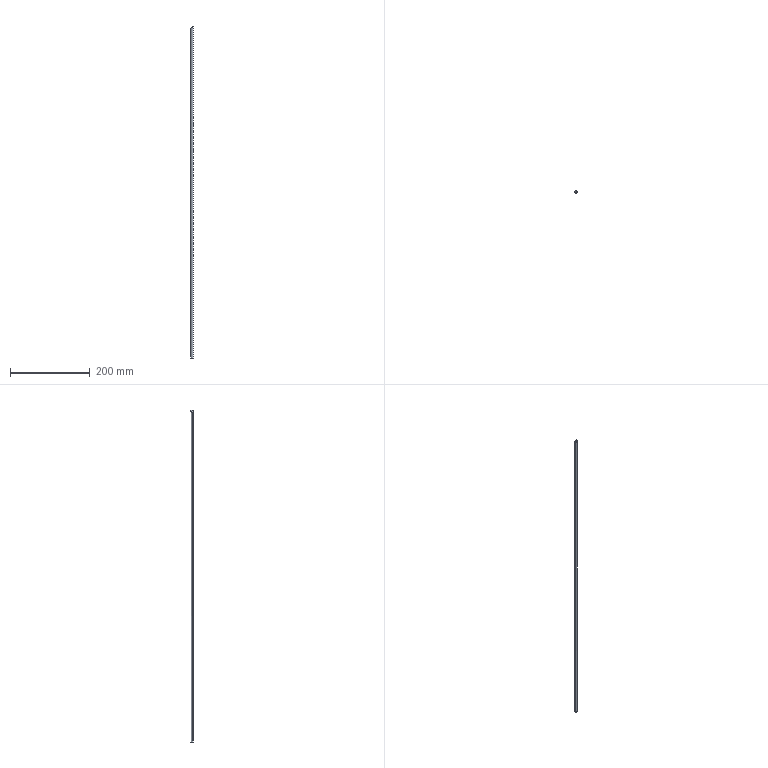Part | SolidWorks | features Extrusion 1, ICE 1 | 1 solid | 4 faces | box 6 x 6 x 832.8 mm | volume 23463 mm3 | cylinder 2 | plane 2 | commonest cylinder face diameters 6 x2
STEP:
#1=CARTESIAN_POINT('',(-3.,0.,826.8));
#2=VERTEX_POINT('',#1);
#3=CARTESIAN_POINT('',(3.,0.,832.8));
#4=VERTEX_POINT('',#3);
#5=CARTESIAN_POINT('',(-3.,0.,826.8));
#6=CARTESIAN_POINT('',(-3.,6.,826.8));
#7=CARTESIAN_POINT('',(3.,6.,832.8));
#8=CARTESIAN_POINT('',(3.,0.,832.8));
#9=(BOUNDED_CURVE()B_SPLINE_CURVE(3,(#5,#6,#7,#8),.UNSPECIFIED.,.F.,.F.)B_SPLINE_CURVE_WITH_KNOTS((4,4),(0.,3.142),.UNSPECIFIED.)CURVE()GEOMETRIC_REPRESENTATION_ITEM()RATIONAL_B_SPLINE_CURVE((1.,0.3333,0.3333,1.))REPRESENTATION_ITEM(''));
#10=EDGE_CURVE('',#2,#4,#9,.T.);
#11=ORIENTED_EDGE('',*,*,#10,.T.);
#12=CARTESIAN_POINT('',(3.,0.,0.));
#13=VERTEX_POINT('',#12);
#14=CARTESIAN_POINT('',(3.,0.,832.8));
#15=DIRECTION('',(0.,0.,-1.));
#16=VECTOR('',#15,1000.);
#17=LINE('',#14,#16);
#18=EDGE_CURVE('',#4,#13,#17,.T.);
#19=ORIENTED_EDGE('',*,*,#18,.T.);
#20=CARTESIAN_POINT('',(-3.,0.,0.));
#21=VERTEX_POINT('',#20);
#22=CARTESIAN_POINT('',(0.,0.,0.));
#23=DIRECTION('',(0.,0.,1.));
#24=DIRECTION('',(1.,0.,0.));
#25=AXIS2_PLACEMENT_3D('',#22,#23,#24);
#26=CIRCLE('',#25,3.);
#27=EDGE_CURVE('',#13,#21,#26,.T.);
#28=ORIENTED_EDGE('',*,*,#27,.T.);
#29=CARTESIAN_POINT('',(-3.,0.,832.8));
#30=DIRECTION('',(0.,0.,-1.));
#31=VECTOR('',#30,1000.);
#32=LINE('',#29,#31);
#33=EDGE_CURVE('',#2,#21,#32,.T.);
#34=ORIENTED_EDGE('',*,*,#33,.F.);
#35=EDGE_LOOP('',(#11,#19,#28,#34));
#36=FACE_OUTER_BOUND('',#35,.T.);
#37=CARTESIAN_POINT('',(0.,0.,832.8));
#38=DIRECTION('',(0.,0.,-1.));
#39=DIRECTION('',(-1.,0.,0.));
#40=AXIS2_PLACEMENT_3D('',#37,#38,#39);
#41=CYLINDRICAL_SURFACE('',#40,3.);
#42=ADVANCED_FACE('',(#36),#41,.T.);
#43=ORIENTED_EDGE('',*,*,#18,.F.);
#44=CARTESIAN_POINT('',(3.,0.,832.8));
#45=CARTESIAN_POINT('',(3.,-6.,832.8));
#46=CARTESIAN_POINT('',(-3.,-6.,826.8));
#47=CARTESIAN_POINT('',(-3.,0.,826.8));
#48=(BOUNDED_CURVE()B_SPLINE_CURVE(3,(#44,#45,#46,#47),.UNSPECIFIED.,.F.,.F.)B_SPLINE_CURVE_WITH_KNOTS((4,4),(3.142,6.283),.UNSPECIFIED.)CURVE()GEOMETRIC_REPRESENTATION_ITEM()RATIONAL_B_SPLINE_CURVE((1.,0.3333,0.3333,1.))REPRESENTATION_ITEM(''));
#49=EDGE_CURVE('',#4,#2,#48,.T.);
#50=ORIENTED_EDGE('',*,*,#49,.T.);
#51=ORIENTED_EDGE('',*,*,#33,.T.);
#52=CARTESIAN_POINT('',(0.,0.,0.));
#53=DIRECTION('',(0.,0.,1.));
#54=DIRECTION('',(1.,0.,0.));
#55=AXIS2_PLACEMENT_3D('',#52,#53,#54);
#56=CIRCLE('',#55,3.);
#57=EDGE_CURVE('',#21,#13,#56,.T.);
#58=ORIENTED_EDGE('',*,*,#57,.T.);
#59=EDGE_LOOP('',(#43,#50,#51,#58));
#60=FACE_OUTER_BOUND('',#59,.T.);
#61=CARTESIAN_POINT('',(0.,0.,832.8));
#62=DIRECTION('',(0.,0.,-1.));
#63=DIRECTION('',(-1.,0.,0.));
#64=AXIS2_PLACEMENT_3D('',#61,#62,#63);
#65=CYLINDRICAL_SURFACE('',#64,3.);
#66=ADVANCED_FACE('',(#60),#65,.T.);
#67=ORIENTED_EDGE('',*,*,#57,.F.);
#68=ORIENTED_EDGE('',*,*,#27,.F.);
#69=EDGE_LOOP('',(#67,#68));
#70=FACE_OUTER_BOUND('',#69,.T.);
#71=CARTESIAN_POINT('',(0.,0.,0.));
#72=DIRECTION('',(0.,0.,1.));
#73=DIRECTION('',(1.,0.,0.));
#74=AXIS2_PLACEMENT_3D('',#71,#72,#73);
#75=PLANE('',#74);
#76=ADVANCED_FACE('',(#70),#75,.F.);
#77=ORIENTED_EDGE('',*,*,#10,.F.);
#78=ORIENTED_EDGE('',*,*,#49,.F.);
#79=EDGE_LOOP('',(#77,#78));
#80=FACE_OUTER_BOUND('',#79,.T.);
#81=CARTESIAN_POINT('',(3.,-3.,832.8));
#82=DIRECTION('',(0.7071,0.,-0.7071));
#83=DIRECTION('',(-0.7071,0.,-0.7071));
#84=AXIS2_PLACEMENT_3D('',#81,#82,#83);
#85=PLANE('',#84);
#86=ADVANCED_FACE('',(#80),#85,.F.);
#87=CLOSED_SHELL('',(#42,#66,#76,#86));
#88=MANIFOLD_SOLID_BREP('',#87);
#89=CARTESIAN_POINT('',(0.,0.,0.));
#90=DIRECTION('',(0.,0.,1.));
#91=DIRECTION('',(1.,0.,0.));
#92=AXIS2_PLACEMENT_3D('',#89,#90,#91);
#93=(LENGTH_UNIT()NAMED_UNIT(*)SI_UNIT(.MILLI.,.METRE.));
#94=UNCERTAINTY_MEASURE_WITH_UNIT(LENGTH_MEASURE(0.00001),#93,'','');
#95=(NAMED_UNIT(*)PLANE_ANGLE_UNIT()SI_UNIT($,.RADIAN.));
#96=(NAMED_UNIT(*)SI_UNIT($,.STERADIAN.)SOLID_ANGLE_UNIT());
#97=(GEOMETRIC_REPRESENTATION_CONTEXT(3)GLOBAL_UNCERTAINTY_ASSIGNED_CONTEXT((#94))GLOBAL_UNIT_ASSIGNED_CONTEXT((#93,#95,#96))REPRESENTATION_CONTEXT('',''));
#98=ADVANCED_BREP_SHAPE_REPRESENTATION('',(#88,#92),#97);